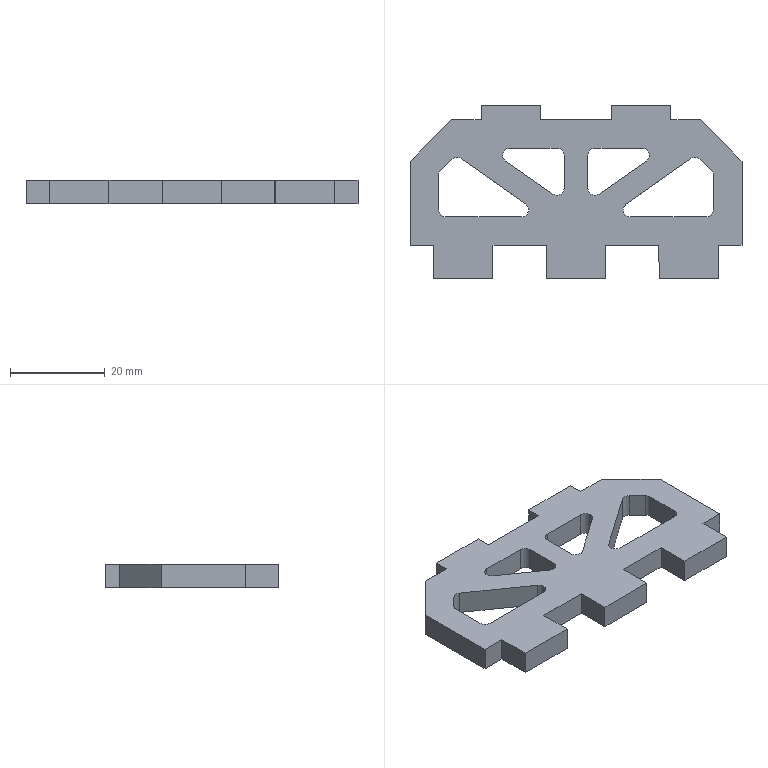Part | SolidWorks | features Fillet 3, Extrusion 1 | 1 solid | 58 faces | box 70 x 36.517 x 5 mm | volume 8161 mm3 | plane 42 | cylinder 16 | commonest cylinder face diameters 3 x16